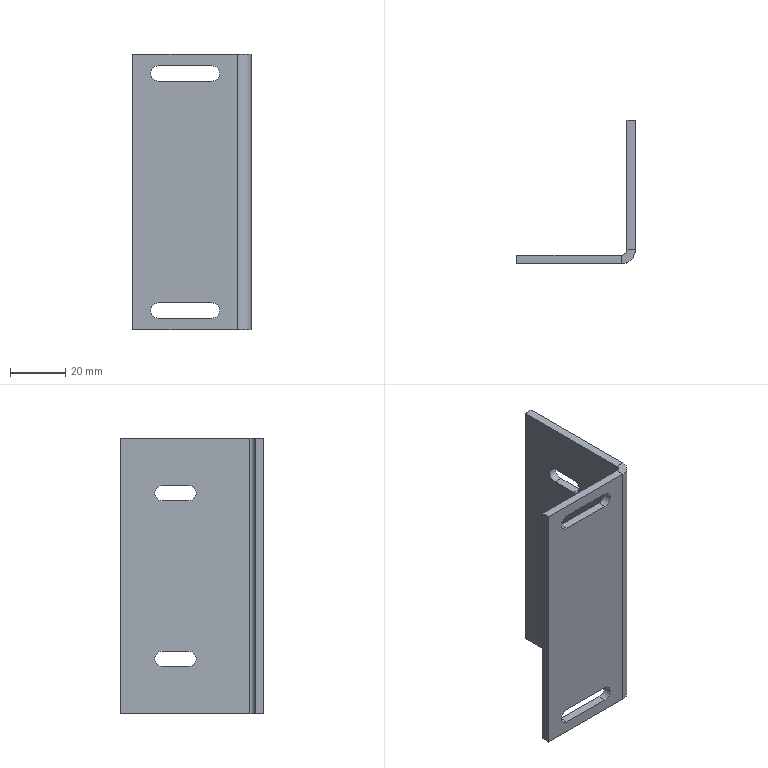Part | SolidWorks | features HoleWzd 2, FlatPattern 1, SMBaseFlange 1, SheetMetal 1 | 1 solid | 30 faces | box 43 x 52 x 100 mm | volume 25907 mm3 | plane 20 | cylinder 10 | commonest cylinder face diameters 5.5 x8 4 x1 10 x1
STEP:
#1=CARTESIAN_POINT('',(40.,2.,100.));
#2=VERTEX_POINT('',#1);
#3=CARTESIAN_POINT('',(43.,2.,100.));
#4=VERTEX_POINT('',#3);
#5=CARTESIAN_POINT('',(40.,2.,100.));
#6=DIRECTION('',(1.,0.,0.));
#7=VECTOR('',#6,1000.);
#8=LINE('',#5,#7);
#9=EDGE_CURVE('',#2,#4,#8,.T.);
#10=ORIENTED_EDGE('',*,*,#9,.F.);
#11=CARTESIAN_POINT('',(38.,0.,100.));
#12=VERTEX_POINT('',#11);
#13=CARTESIAN_POINT('',(38.,2.,100.));
#14=DIRECTION('',(0.,0.,1.));
#15=DIRECTION('',(-1.,0.,0.));
#16=AXIS2_PLACEMENT_3D('',#13,#14,#15);
#17=CIRCLE('',#16,2.);
#18=EDGE_CURVE('',#12,#2,#17,.T.);
#19=ORIENTED_EDGE('',*,*,#18,.F.);
#20=CARTESIAN_POINT('',(38.,-3.,100.));
#21=VERTEX_POINT('',#20);
#22=CARTESIAN_POINT('',(38.,-3.,100.));
#23=DIRECTION('',(0.,1.,0.));
#24=VECTOR('',#23,1000.);
#25=LINE('',#22,#24);
#26=EDGE_CURVE('',#21,#12,#25,.T.);
#27=ORIENTED_EDGE('',*,*,#26,.F.);
#28=CARTESIAN_POINT('',(38.,2.,100.));
#29=DIRECTION('',(0.,0.,1.));
#30=DIRECTION('',(1.,0.,0.));
#31=AXIS2_PLACEMENT_3D('',#28,#29,#30);
#32=CIRCLE('',#31,5.);
#33=EDGE_CURVE('',#21,#4,#32,.T.);
#34=ORIENTED_EDGE('',*,*,#33,.T.);
#35=EDGE_LOOP('',(#10,#19,#27,#34));
#36=FACE_OUTER_BOUND('',#35,.T.);
#37=CARTESIAN_POINT('',(40.,2.,100.));
#38=DIRECTION('',(0.,0.,1.));
#39=DIRECTION('',(1.,0.,0.));
#40=AXIS2_PLACEMENT_3D('',#37,#38,#39);
#41=PLANE('',#40);
#42=ADVANCED_FACE('',(#36),#41,.T.);
#43=CARTESIAN_POINT('',(40.,49.,100.));
#44=VERTEX_POINT('',#43);
#45=CARTESIAN_POINT('',(40.,0.,100.));
#46=DIRECTION('',(0.,1.,0.));
#47=VECTOR('',#46,1000.);
#48=LINE('',#45,#47);
#49=EDGE_CURVE('',#2,#44,#48,.T.);
#50=ORIENTED_EDGE('',*,*,#49,.F.);
#51=ORIENTED_EDGE('',*,*,#9,.T.);
#52=CARTESIAN_POINT('',(43.,49.,100.));
#53=VERTEX_POINT('',#52);
#54=CARTESIAN_POINT('',(43.,0.,100.));
#55=DIRECTION('',(0.,1.,0.));
#56=VECTOR('',#55,1000.);
#57=LINE('',#54,#56);
#58=EDGE_CURVE('',#4,#53,#57,.T.);
#59=ORIENTED_EDGE('',*,*,#58,.T.);
#60=CARTESIAN_POINT('',(40.,49.,100.));
#61=DIRECTION('',(1.,0.,0.));
#62=VECTOR('',#61,1000.);
#63=LINE('',#60,#62);
#64=EDGE_CURVE('',#44,#53,#63,.T.);
#65=ORIENTED_EDGE('',*,*,#64,.F.);
#66=EDGE_LOOP('',(#50,#51,#59,#65));
#67=FACE_OUTER_BOUND('',#66,.T.);
#68=CARTESIAN_POINT('',(38.,-3.,100.));
#69=DIRECTION('',(0.,0.,1.));
#70=DIRECTION('',(1.,0.,0.));
#71=AXIS2_PLACEMENT_3D('',#68,#69,#70);
#72=PLANE('',#71);
#73=ADVANCED_FACE('',(#67),#72,.T.);
#74=CARTESIAN_POINT('',(38.,0.,0.));
#75=VERTEX_POINT('',#74);
#76=CARTESIAN_POINT('',(38.,-3.,0.));
#77=VERTEX_POINT('',#76);
#78=CARTESIAN_POINT('',(38.,0.,0.));
#79=DIRECTION('',(0.,-1.,0.));
#80=VECTOR('',#79,1000.);
#81=LINE('',#78,#80);
#82=EDGE_CURVE('',#75,#77,#81,.T.);
#83=ORIENTED_EDGE('',*,*,#82,.F.);
#84=CARTESIAN_POINT('',(40.,2.,0.));
#85=VERTEX_POINT('',#84);
#86=CARTESIAN_POINT('',(38.,2.,0.));
#87=DIRECTION('',(0.,0.,1.));
#88=DIRECTION('',(-1.,0.,0.));
#89=AXIS2_PLACEMENT_3D('',#86,#87,#88);
#90=CIRCLE('',#89,2.);
#91=EDGE_CURVE('',#75,#85,#90,.T.);
#92=ORIENTED_EDGE('',*,*,#91,.T.);
#93=CARTESIAN_POINT('',(43.,2.,0.));
#94=VERTEX_POINT('',#93);
#95=CARTESIAN_POINT('',(43.,2.,0.));
#96=DIRECTION('',(-1.,0.,0.));
#97=VECTOR('',#96,1000.);
#98=LINE('',#95,#97);
#99=EDGE_CURVE('',#94,#85,#98,.T.);
#100=ORIENTED_EDGE('',*,*,#99,.F.);
#101=CARTESIAN_POINT('',(38.,2.,0.));
#102=DIRECTION('',(0.,0.,1.));
#103=DIRECTION('',(1.,0.,0.));
#104=AXIS2_PLACEMENT_3D('',#101,#102,#103);
#105=CIRCLE('',#104,5.);
#106=EDGE_CURVE('',#77,#94,#105,.T.);
#107=ORIENTED_EDGE('',*,*,#106,.F.);
#108=EDGE_LOOP('',(#83,#92,#100,#107));
#109=FACE_OUTER_BOUND('',#108,.T.);
#110=CARTESIAN_POINT('',(38.,0.,0.));
#111=DIRECTION('',(0.,0.,-1.));
#112=DIRECTION('',(-1.,0.,0.));
#113=AXIS2_PLACEMENT_3D('',#110,#111,#112);
#114=PLANE('',#113);
#115=ADVANCED_FACE('',(#109),#114,.T.);
#116=CARTESIAN_POINT('',(0.,0.,0.));
#117=VERTEX_POINT('',#116);
#118=CARTESIAN_POINT('',(0.,0.,0.));
#119=DIRECTION('',(1.,0.,0.));
#120=VECTOR('',#119,1000.);
#121=LINE('',#118,#120);
#122=EDGE_CURVE('',#117,#75,#121,.T.);
#123=ORIENTED_EDGE('',*,*,#122,.T.);
#124=ORIENTED_EDGE('',*,*,#82,.T.);
#125=CARTESIAN_POINT('',(0.,-3.,0.));
#126=VERTEX_POINT('',#125);
#127=CARTESIAN_POINT('',(0.,-3.,0.));
#128=DIRECTION('',(1.,0.,0.));
#129=VECTOR('',#128,1000.);
#130=LINE('',#127,#129);
#131=EDGE_CURVE('',#126,#77,#130,.T.);
#132=ORIENTED_EDGE('',*,*,#131,.F.);
#133=CARTESIAN_POINT('',(0.,-3.,0.));
#134=DIRECTION('',(0.,1.,0.));
#135=VECTOR('',#134,1000.);
#136=LINE('',#133,#135);
#137=EDGE_CURVE('',#126,#117,#136,.T.);
#138=ORIENTED_EDGE('',*,*,#137,.T.);
#139=EDGE_LOOP('',(#123,#124,#132,#138));
#140=FACE_OUTER_BOUND('',#139,.T.);
#141=CARTESIAN_POINT('',(43.,2.,0.));
#142=DIRECTION('',(0.,0.,-1.));
#143=DIRECTION('',(-1.,0.,0.));
#144=AXIS2_PLACEMENT_3D('',#141,#142,#143);
#145=PLANE('',#144);
#146=ADVANCED_FACE('',(#140),#145,.T.);
#147=CARTESIAN_POINT('',(43.,24.25,17.25));
#148=VERTEX_POINT('',#147);
#149=CARTESIAN_POINT('',(43.,24.25,22.75));
#150=VERTEX_POINT('',#149);
#151=CARTESIAN_POINT('',(43.,24.25,20.));
#152=DIRECTION('',(-1.,0.,0.));
#153=DIRECTION('',(0.,0.,1.));
#154=AXIS2_PLACEMENT_3D('',#151,#152,#153);
#155=CIRCLE('',#154,2.75);
#156=EDGE_CURVE('',#148,#150,#155,.T.);
#157=ORIENTED_EDGE('',*,*,#156,.T.);
#158=CARTESIAN_POINT('',(43.,33.75,22.75));
#159=VERTEX_POINT('',#158);
#160=CARTESIAN_POINT('',(43.,24.25,22.75));
#161=DIRECTION('',(0.,1.,0.));
#162=VECTOR('',#161,1000.);
#163=LINE('',#160,#162);
#164=EDGE_CURVE('',#150,#159,#163,.T.);
#165=ORIENTED_EDGE('',*,*,#164,.T.);
#166=CARTESIAN_POINT('',(43.,33.75,17.25));
#167=VERTEX_POINT('',#166);
#168=CARTESIAN_POINT('',(43.,33.75,20.));
#169=DIRECTION('',(-1.,0.,0.));
#170=DIRECTION('',(0.,0.,1.));
#171=AXIS2_PLACEMENT_3D('',#168,#169,#170);
#172=CIRCLE('',#171,2.75);
#173=EDGE_CURVE('',#159,#167,#172,.T.);
#174=ORIENTED_EDGE('',*,*,#173,.T.);
#175=CARTESIAN_POINT('',(43.,24.25,17.25));
#176=DIRECTION('',(0.,1.,0.));
#177=VECTOR('',#176,1000.);
#178=LINE('',#175,#177);
#179=EDGE_CURVE('',#148,#167,#178,.T.);
#180=ORIENTED_EDGE('',*,*,#179,.F.);
#181=EDGE_LOOP('',(#157,#165,#174,#180));
#182=FACE_BOUND('',#181,.T.);
#183=CARTESIAN_POINT('',(43.,33.75,82.75));
#184=VERTEX_POINT('',#183);
#185=CARTESIAN_POINT('',(43.,33.75,77.25));
#186=VERTEX_POINT('',#185);
#187=CARTESIAN_POINT('',(43.,33.75,80.));
#188=DIRECTION('',(-1.,0.,0.));
#189=DIRECTION('',(0.,0.,1.));
#190=AXIS2_PLACEMENT_3D('',#187,#188,#189);
#191=CIRCLE('',#190,2.75);
#192=EDGE_CURVE('',#184,#186,#191,.T.);
#193=ORIENTED_EDGE('',*,*,#192,.T.);
#194=CARTESIAN_POINT('',(43.,24.25,77.25));
#195=VERTEX_POINT('',#194);
#196=CARTESIAN_POINT('',(43.,24.25,77.25));
#197=DIRECTION('',(0.,1.,0.));
#198=VECTOR('',#197,1000.);
#199=LINE('',#196,#198);
#200=EDGE_CURVE('',#195,#186,#199,.T.);
#201=ORIENTED_EDGE('',*,*,#200,.F.);
#202=CARTESIAN_POINT('',(43.,24.25,82.75));
#203=VERTEX_POINT('',#202);
#204=CARTESIAN_POINT('',(43.,24.25,80.));
#205=DIRECTION('',(-1.,0.,0.));
#206=DIRECTION('',(0.,0.,1.));
#207=AXIS2_PLACEMENT_3D('',#204,#205,#206);
#208=CIRCLE('',#207,2.75);
#209=EDGE_CURVE('',#195,#203,#208,.T.);
#210=ORIENTED_EDGE('',*,*,#209,.T.);
#211=CARTESIAN_POINT('',(43.,24.25,82.75));
#212=DIRECTION('',(0.,1.,0.));
#213=VECTOR('',#212,1000.);
#214=LINE('',#211,#213);
#215=EDGE_CURVE('',#203,#184,#214,.T.);
#216=ORIENTED_EDGE('',*,*,#215,.T.);
#217=EDGE_LOOP('',(#193,#201,#210,#216));
#218=FACE_BOUND('',#217,.T.);
#219=CARTESIAN_POINT('',(43.,49.,0.));
#220=VERTEX_POINT('',#219);
#221=CARTESIAN_POINT('',(43.,0.,0.));
#222=DIRECTION('',(0.,1.,0.));
#223=VECTOR('',#222,1000.);
#224=LINE('',#221,#223);
#225=EDGE_CURVE('',#94,#220,#224,.T.);
#226=ORIENTED_EDGE('',*,*,#225,.T.);
#227=CARTESIAN_POINT('',(43.,49.,100.));
#228=DIRECTION('',(0.,0.,-1.));
#229=VECTOR('',#228,1000.);
#230=LINE('',#227,#229);
#231=EDGE_CURVE('',#53,#220,#230,.T.);
#232=ORIENTED_EDGE('',*,*,#231,.F.);
#233=ORIENTED_EDGE('',*,*,#58,.F.);
#234=CARTESIAN_POINT('',(43.,2.,100.));
#235=DIRECTION('',(0.,0.,-1.));
#236=VECTOR('',#235,1000.);
#237=LINE('',#234,#236);
#238=EDGE_CURVE('',#4,#94,#237,.T.);
#239=ORIENTED_EDGE('',*,*,#238,.T.);
#240=EDGE_LOOP('',(#226,#232,#233,#239));
#241=FACE_OUTER_BOUND('',#240,.T.);
#242=CARTESIAN_POINT('',(43.,0.,100.));
#243=DIRECTION('',(-1.,0.,0.));
#244=DIRECTION('',(0.,0.,1.));
#245=AXIS2_PLACEMENT_3D('',#242,#243,#244);
#246=PLANE('',#245);
#247=ADVANCED_FACE('',(#182,#218,#241),#246,.F.);
#248=CARTESIAN_POINT('',(40.,49.,0.));
#249=VERTEX_POINT('',#248);
#250=CARTESIAN_POINT('',(40.,49.,0.));
#251=DIRECTION('',(1.,0.,0.));
#252=VECTOR('',#251,1000.);
#253=LINE('',#250,#252);
#254=EDGE_CURVE('',#249,#220,#253,.T.);
#255=ORIENTED_EDGE('',*,*,#254,.F.);
#256=CARTESIAN_POINT('',(40.,49.,100.));
#257=DIRECTION('',(0.,0.,-1.));
#258=VECTOR('',#257,1000.);
#259=LINE('',#256,#258);
#260=EDGE_CURVE('',#44,#249,#259,.T.);
#261=ORIENTED_EDGE('',*,*,#260,.F.);
#262=ORIENTED_EDGE('',*,*,#64,.T.);
#263=ORIENTED_EDGE('',*,*,#231,.T.);
#264=EDGE_LOOP('',(#255,#261,#262,#263));
#265=FACE_OUTER_BOUND('',#264,.T.);
#266=CARTESIAN_POINT('',(40.,49.,100.));
#267=DIRECTION('',(0.,1.,0.));
#268=DIRECTION('',(0.,0.,1.));
#269=AXIS2_PLACEMENT_3D('',#266,#267,#268);
#270=PLANE('',#269);
#271=ADVANCED_FACE('',(#265),#270,.T.);
#272=CARTESIAN_POINT('',(40.,33.75,22.75));
#273=VERTEX_POINT('',#272);
#274=CARTESIAN_POINT('',(40.,33.75,17.25));
#275=VERTEX_POINT('',#274);
#276=CARTESIAN_POINT('',(40.,33.75,20.));
#277=DIRECTION('',(-1.,0.,0.));
#278=DIRECTION('',(0.,0.,1.));
#279=AXIS2_PLACEMENT_3D('',#276,#277,#278);
#280=CIRCLE('',#279,2.75);
#281=EDGE_CURVE('',#273,#275,#280,.T.);
#282=ORIENTED_EDGE('',*,*,#281,.F.);
#283=CARTESIAN_POINT('',(40.,24.25,22.75));
#284=VERTEX_POINT('',#283);
#285=CARTESIAN_POINT('',(40.,24.25,22.75));
#286=DIRECTION('',(0.,1.,0.));
#287=VECTOR('',#286,1000.);
#288=LINE('',#285,#287);
#289=EDGE_CURVE('',#284,#273,#288,.T.);
#290=ORIENTED_EDGE('',*,*,#289,.F.);
#291=CARTESIAN_POINT('',(40.,24.25,17.25));
#292=VERTEX_POINT('',#291);
#293=CARTESIAN_POINT('',(40.,24.25,20.));
#294=DIRECTION('',(-1.,0.,0.));
#295=DIRECTION('',(0.,0.,1.));
#296=AXIS2_PLACEMENT_3D('',#293,#294,#295);
#297=CIRCLE('',#296,2.75);
#298=EDGE_CURVE('',#292,#284,#297,.T.);
#299=ORIENTED_EDGE('',*,*,#298,.F.);
#300=CARTESIAN_POINT('',(40.,24.25,17.25));
#301=DIRECTION('',(0.,1.,0.));
#302=VECTOR('',#301,1000.);
#303=LINE('',#300,#302);
#304=EDGE_CURVE('',#292,#275,#303,.T.);
#305=ORIENTED_EDGE('',*,*,#304,.T.);
#306=EDGE_LOOP('',(#282,#290,#299,#305));
#307=FACE_BOUND('',#306,.T.);
#308=CARTESIAN_POINT('',(40.,33.75,82.75));
#309=VERTEX_POINT('',#308);
#310=CARTESIAN_POINT('',(40.,33.75,77.25));
#311=VERTEX_POINT('',#310);
#312=CARTESIAN_POINT('',(40.,33.75,80.));
#313=DIRECTION('',(-1.,0.,0.));
#314=DIRECTION('',(0.,0.,1.));
#315=AXIS2_PLACEMENT_3D('',#312,#313,#314);
#316=CIRCLE('',#315,2.75);
#317=EDGE_CURVE('',#309,#311,#316,.T.);
#318=ORIENTED_EDGE('',*,*,#317,.F.);
#319=CARTESIAN_POINT('',(40.,24.25,82.75));
#320=VERTEX_POINT('',#319);
#321=CARTESIAN_POINT('',(40.,24.25,82.75));
#322=DIRECTION('',(0.,1.,0.));
#323=VECTOR('',#322,1000.);
#324=LINE('',#321,#323);
#325=EDGE_CURVE('',#320,#309,#324,.T.);
#326=ORIENTED_EDGE('',*,*,#325,.F.);
#327=CARTESIAN_POINT('',(40.,24.25,77.25));
#328=VERTEX_POINT('',#327);
#329=CARTESIAN_POINT('',(40.,24.25,80.));
#330=DIRECTION('',(-1.,0.,0.));
#331=DIRECTION('',(0.,0.,1.));
#332=AXIS2_PLACEMENT_3D('',#329,#330,#331);
#333=CIRCLE('',#332,2.75);
#334=EDGE_CURVE('',#328,#320,#333,.T.);
#335=ORIENTED_EDGE('',*,*,#334,.F.);
#336=CARTESIAN_POINT('',(40.,24.25,77.25));
#337=DIRECTION('',(0.,1.,0.));
#338=VECTOR('',#337,1000.);
#339=LINE('',#336,#338);
#340=EDGE_CURVE('',#328,#311,#339,.T.);
#341=ORIENTED_EDGE('',*,*,#340,.T.);
#342=EDGE_LOOP('',(#318,#326,#335,#341));
#343=FACE_BOUND('',#342,.T.);
#344=CARTESIAN_POINT('',(40.,0.,0.));
#345=DIRECTION('',(0.,1.,0.));
#346=VECTOR('',#345,1000.);
#347=LINE('',#344,#346);
#348=EDGE_CURVE('',#85,#249,#347,.T.);
#349=ORIENTED_EDGE('',*,*,#348,.F.);
#350=CARTESIAN_POINT('',(40.,2.,100.));
#351=DIRECTION('',(0.,0.,-1.));
#352=VECTOR('',#351,1000.);
#353=LINE('',#350,#352);
#354=EDGE_CURVE('',#2,#85,#353,.T.);
#355=ORIENTED_EDGE('',*,*,#354,.F.);
#356=ORIENTED_EDGE('',*,*,#49,.T.);
#357=ORIENTED_EDGE('',*,*,#260,.T.);
#358=EDGE_LOOP('',(#349,#355,#356,#357));
#359=FACE_OUTER_BOUND('',#358,.T.);
#360=CARTESIAN_POINT('',(40.,0.,100.));
#361=DIRECTION('',(-1.,0.,0.));
#362=DIRECTION('',(0.,0.,1.));
#363=AXIS2_PLACEMENT_3D('',#360,#361,#362);
#364=PLANE('',#363);
#365=ADVANCED_FACE('',(#307,#343,#359),#364,.T.);
#366=ORIENTED_EDGE('',*,*,#91,.F.);
#367=CARTESIAN_POINT('',(38.,0.,100.));
#368=DIRECTION('',(0.,0.,-1.));
#369=VECTOR('',#368,1000.);
#370=LINE('',#367,#369);
#371=EDGE_CURVE('',#12,#75,#370,.T.);
#372=ORIENTED_EDGE('',*,*,#371,.F.);
#373=ORIENTED_EDGE('',*,*,#18,.T.);
#374=ORIENTED_EDGE('',*,*,#354,.T.);
#375=EDGE_LOOP('',(#366,#372,#373,#374));
#376=FACE_OUTER_BOUND('',#375,.T.);
#377=CARTESIAN_POINT('',(38.,2.,100.));
#378=DIRECTION('',(0.,0.,-1.));
#379=DIRECTION('',(-1.,0.,0.));
#380=AXIS2_PLACEMENT_3D('',#377,#378,#379);
#381=CYLINDRICAL_SURFACE('',#380,2.);
#382=ADVANCED_FACE('',(#376),#381,.F.);
#383=CARTESIAN_POINT('',(9.25,0.,9.75));
#384=VERTEX_POINT('',#383);
#385=CARTESIAN_POINT('',(28.75,0.,9.75));
#386=VERTEX_POINT('',#385);
#387=CARTESIAN_POINT('',(9.25,0.,9.75));
#388=DIRECTION('',(1.,0.,0.));
#389=VECTOR('',#388,1000.);
#390=LINE('',#387,#389);
#391=EDGE_CURVE('',#384,#386,#390,.T.);
#392=ORIENTED_EDGE('',*,*,#391,.F.);
#393=CARTESIAN_POINT('',(9.25,0.,4.25));
#394=VERTEX_POINT('',#393);
#395=CARTESIAN_POINT('',(9.25,0.,7.));
#396=DIRECTION('',(0.,1.,0.));
#397=DIRECTION('',(0.,0.,1.));
#398=AXIS2_PLACEMENT_3D('',#395,#396,#397);
#399=CIRCLE('',#398,2.75);
#400=EDGE_CURVE('',#394,#384,#399,.T.);
#401=ORIENTED_EDGE('',*,*,#400,.F.);
#402=CARTESIAN_POINT('',(28.75,0.,4.25));
#403=VERTEX_POINT('',#402);
#404=CARTESIAN_POINT('',(9.25,0.,4.25));
#405=DIRECTION('',(1.,0.,0.));
#406=VECTOR('',#405,1000.);
#407=LINE('',#404,#406);
#408=EDGE_CURVE('',#394,#403,#407,.T.);
#409=ORIENTED_EDGE('',*,*,#408,.T.);
#410=CARTESIAN_POINT('',(28.75,0.,7.));
#411=DIRECTION('',(0.,1.,0.));
#412=DIRECTION('',(0.,0.,1.));
#413=AXIS2_PLACEMENT_3D('',#410,#411,#412);
#414=CIRCLE('',#413,2.75);
#415=EDGE_CURVE('',#386,#403,#414,.T.);
#416=ORIENTED_EDGE('',*,*,#415,.F.);
#417=EDGE_LOOP('',(#392,#401,#409,#416));
#418=FACE_BOUND('',#417,.T.);
#419=CARTESIAN_POINT('',(9.25,0.,90.25));
#420=VERTEX_POINT('',#419);
#421=CARTESIAN_POINT('',(9.25,0.,95.75));
#422=VERTEX_POINT('',#421);
#423=CARTESIAN_POINT('',(9.25,0.,93.));
#424=DIRECTION('',(0.,1.,0.));
#425=DIRECTION('',(0.,0.,1.));
#426=AXIS2_PLACEMENT_3D('',#423,#424,#425);
#427=CIRCLE('',#426,2.75);
#428=EDGE_CURVE('',#420,#422,#427,.T.);
#429=ORIENTED_EDGE('',*,*,#428,.F.);
#430=CARTESIAN_POINT('',(28.75,0.,90.25));
#431=VERTEX_POINT('',#430);
#432=CARTESIAN_POINT('',(9.25,0.,90.25));
#433=DIRECTION('',(1.,0.,0.));
#434=VECTOR('',#433,1000.);
#435=LINE('',#432,#434);
#436=EDGE_CURVE('',#420,#431,#435,.T.);
#437=ORIENTED_EDGE('',*,*,#436,.T.);
#438=CARTESIAN_POINT('',(28.75,0.,95.75));
#439=VERTEX_POINT('',#438);
#440=CARTESIAN_POINT('',(28.75,0.,93.));
#441=DIRECTION('',(0.,1.,0.));
#442=DIRECTION('',(0.,0.,1.));
#443=AXIS2_PLACEMENT_3D('',#440,#441,#442);
#444=CIRCLE('',#443,2.75);
#445=EDGE_CURVE('',#439,#431,#444,.T.);
#446=ORIENTED_EDGE('',*,*,#445,.F.);
#447=CARTESIAN_POINT('',(9.25,0.,95.75));
#448=DIRECTION('',(1.,0.,0.));
#449=VECTOR('',#448,1000.);
#450=LINE('',#447,#449);
#451=EDGE_CURVE('',#422,#439,#450,.T.);
#452=ORIENTED_EDGE('',*,*,#451,.F.);
#453=EDGE_LOOP('',(#429,#437,#446,#452));
#454=FACE_BOUND('',#453,.T.);
#455=ORIENTED_EDGE('',*,*,#122,.F.);
#456=CARTESIAN_POINT('',(0.,0.,100.));
#457=VERTEX_POINT('',#456);
#458=CARTESIAN_POINT('',(0.,0.,100.));
#459=DIRECTION('',(0.,0.,-1.));
#460=VECTOR('',#459,1000.);
#461=LINE('',#458,#460);
#462=EDGE_CURVE('',#457,#117,#461,.T.);
#463=ORIENTED_EDGE('',*,*,#462,.F.);
#464=CARTESIAN_POINT('',(0.,0.,100.));
#465=DIRECTION('',(1.,0.,0.));
#466=VECTOR('',#465,1000.);
#467=LINE('',#464,#466);
#468=EDGE_CURVE('',#457,#12,#467,.T.);
#469=ORIENTED_EDGE('',*,*,#468,.T.);
#470=ORIENTED_EDGE('',*,*,#371,.T.);
#471=EDGE_LOOP('',(#455,#463,#469,#470));
#472=FACE_OUTER_BOUND('',#471,.T.);
#473=CARTESIAN_POINT('',(0.,0.,100.));
#474=DIRECTION('',(0.,1.,0.));
#475=DIRECTION('',(0.,0.,1.));
#476=AXIS2_PLACEMENT_3D('',#473,#474,#475);
#477=PLANE('',#476);
#478=ADVANCED_FACE('',(#418,#454,#472),#477,.T.);
#479=ORIENTED_EDGE('',*,*,#137,.F.);
#480=CARTESIAN_POINT('',(0.,-3.,100.));
#481=VERTEX_POINT('',#480);
#482=CARTESIAN_POINT('',(0.,-3.,100.));
#483=DIRECTION('',(0.,0.,-1.));
#484=VECTOR('',#483,1000.);
#485=LINE('',#482,#484);
#486=EDGE_CURVE('',#481,#126,#485,.T.);
#487=ORIENTED_EDGE('',*,*,#486,.F.);
#488=CARTESIAN_POINT('',(0.,-3.,100.));
#489=DIRECTION('',(0.,1.,0.));
#490=VECTOR('',#489,1000.);
#491=LINE('',#488,#490);
#492=EDGE_CURVE('',#481,#457,#491,.T.);
#493=ORIENTED_EDGE('',*,*,#492,.T.);
#494=ORIENTED_EDGE('',*,*,#462,.T.);
#495=EDGE_LOOP('',(#479,#487,#493,#494));
#496=FACE_OUTER_BOUND('',#495,.T.);
#497=CARTESIAN_POINT('',(0.,-3.,100.));
#498=DIRECTION('',(-1.,0.,0.));
#499=DIRECTION('',(0.,0.,1.));
#500=AXIS2_PLACEMENT_3D('',#497,#498,#499);
#501=PLANE('',#500);
#502=ADVANCED_FACE('',(#496),#501,.T.);
#503=CARTESIAN_POINT('',(9.25,-3.,9.75));
#504=VERTEX_POINT('',#503);
#505=CARTESIAN_POINT('',(28.75,-3.,9.75));
#506=VERTEX_POINT('',#505);
#507=CARTESIAN_POINT('',(9.25,-3.,9.75));
#508=DIRECTION('',(1.,0.,0.));
#509=VECTOR('',#508,1000.);
#510=LINE('',#507,#509);
#511=EDGE_CURVE('',#504,#506,#510,.T.);
#512=ORIENTED_EDGE('',*,*,#511,.T.);
#513=CARTESIAN_POINT('',(28.75,-3.,4.25));
#514=VERTEX_POINT('',#513);
#515=CARTESIAN_POINT('',(28.75,-3.,7.));
#516=DIRECTION('',(0.,1.,0.));
#517=DIRECTION('',(0.,0.,1.));
#518=AXIS2_PLACEMENT_3D('',#515,#516,#517);
#519=CIRCLE('',#518,2.75);
#520=EDGE_CURVE('',#506,#514,#519,.T.);
#521=ORIENTED_EDGE('',*,*,#520,.T.);
#522=CARTESIAN_POINT('',(9.25,-3.,4.25));
#523=VERTEX_POINT('',#522);
#524=CARTESIAN_POINT('',(9.25,-3.,4.25));
#525=DIRECTION('',(1.,0.,0.));
#526=VECTOR('',#525,1000.);
#527=LINE('',#524,#526);
#528=EDGE_CURVE('',#523,#514,#527,.T.);
#529=ORIENTED_EDGE('',*,*,#528,.F.);
#530=CARTESIAN_POINT('',(9.25,-3.,7.));
#531=DIRECTION('',(0.,1.,0.));
#532=DIRECTION('',(0.,0.,1.));
#533=AXIS2_PLACEMENT_3D('',#530,#531,#532);
#534=CIRCLE('',#533,2.75);
#535=EDGE_CURVE('',#523,#504,#534,.T.);
#536=ORIENTED_EDGE('',*,*,#535,.T.);
#537=EDGE_LOOP('',(#512,#521,#529,#536));
#538=FACE_BOUND('',#537,.T.);
#539=CARTESIAN_POINT('',(9.25,-3.,90.25));
#540=VERTEX_POINT('',#539);
#541=CARTESIAN_POINT('',(9.25,-3.,95.75));
#542=VERTEX_POINT('',#541);
#543=CARTESIAN_POINT('',(9.25,-3.,93.));
#544=DIRECTION('',(0.,1.,0.));
#545=DIRECTION('',(0.,0.,1.));
#546=AXIS2_PLACEMENT_3D('',#543,#544,#545);
#547=CIRCLE('',#546,2.75);
#548=EDGE_CURVE('',#540,#542,#547,.T.);
#549=ORIENTED_EDGE('',*,*,#548,.T.);
#550=CARTESIAN_POINT('',(28.75,-3.,95.75));
#551=VERTEX_POINT('',#550);
#552=CARTESIAN_POINT('',(9.25,-3.,95.75));
#553=DIRECTION('',(1.,0.,0.));
#554=VECTOR('',#553,1000.);
#555=LINE('',#552,#554);
#556=EDGE_CURVE('',#542,#551,#555,.T.);
#557=ORIENTED_EDGE('',*,*,#556,.T.);
#558=CARTESIAN_POINT('',(28.75,-3.,90.25));
#559=VERTEX_POINT('',#558);
#560=CARTESIAN_POINT('',(28.75,-3.,93.));
#561=DIRECTION('',(0.,1.,0.));
#562=DIRECTION('',(0.,0.,1.));
#563=AXIS2_PLACEMENT_3D('',#560,#561,#562);
#564=CIRCLE('',#563,2.75);
#565=EDGE_CURVE('',#551,#559,#564,.T.);
#566=ORIENTED_EDGE('',*,*,#565,.T.);
#567=CARTESIAN_POINT('',(9.25,-3.,90.25));
#568=DIRECTION('',(1.,0.,0.));
#569=VECTOR('',#568,1000.);
#570=LINE('',#567,#569);
#571=EDGE_CURVE('',#540,#559,#570,.T.);
#572=ORIENTED_EDGE('',*,*,#571,.F.);
#573=EDGE_LOOP('',(#549,#557,#566,#572));
#574=FACE_BOUND('',#573,.T.);
#575=ORIENTED_EDGE('',*,*,#131,.T.);
#576=CARTESIAN_POINT('',(38.,-3.,100.));
#577=DIRECTION('',(0.,0.,-1.));
#578=VECTOR('',#577,1000.);
#579=LINE('',#576,#578);
#580=EDGE_CURVE('',#21,#77,#579,.T.);
#581=ORIENTED_EDGE('',*,*,#580,.F.);
#582=CARTESIAN_POINT('',(0.,-3.,100.));
#583=DIRECTION('',(1.,0.,0.));
#584=VECTOR('',#583,1000.);
#585=LINE('',#582,#584);
#586=EDGE_CURVE('',#481,#21,#585,.T.);
#587=ORIENTED_EDGE('',*,*,#586,.F.);
#588=ORIENTED_EDGE('',*,*,#486,.T.);
#589=EDGE_LOOP('',(#575,#581,#587,#588));
#590=FACE_OUTER_BOUND('',#589,.T.);
#591=CARTESIAN_POINT('',(0.,-3.,100.));
#592=DIRECTION('',(0.,1.,0.));
#593=DIRECTION('',(0.,0.,1.));
#594=AXIS2_PLACEMENT_3D('',#591,#592,#593);
#595=PLANE('',#594);
#596=ADVANCED_FACE('',(#538,#574,#590),#595,.F.);
#597=ORIENTED_EDGE('',*,*,#106,.T.);
#598=ORIENTED_EDGE('',*,*,#238,.F.);
#599=ORIENTED_EDGE('',*,*,#33,.F.);
#600=ORIENTED_EDGE('',*,*,#580,.T.);
#601=EDGE_LOOP('',(#597,#598,#599,#600));
#602=FACE_OUTER_BOUND('',#601,.T.);
#603=CARTESIAN_POINT('',(38.,2.,100.));
#604=DIRECTION('',(0.,0.,-1.));
#605=DIRECTION('',(-1.,0.,0.));
#606=AXIS2_PLACEMENT_3D('',#603,#604,#605);
#607=CYLINDRICAL_SURFACE('',#606,5.);
#608=ADVANCED_FACE('',(#602),#607,.T.);
#609=ORIENTED_EDGE('',*,*,#586,.T.);
#610=ORIENTED_EDGE('',*,*,#26,.T.);
#611=ORIENTED_EDGE('',*,*,#468,.F.);
#612=ORIENTED_EDGE('',*,*,#492,.F.);
#613=EDGE_LOOP('',(#609,#610,#611,#612));
#614=FACE_OUTER_BOUND('',#613,.T.);
#615=CARTESIAN_POINT('',(38.,2.,100.));
#616=DIRECTION('',(0.,0.,-1.));
#617=DIRECTION('',(-1.,0.,0.));
#618=AXIS2_PLACEMENT_3D('',#615,#616,#617);
#619=PLANE('',#618);
#620=ADVANCED_FACE('',(#614),#619,.F.);
#621=ORIENTED_EDGE('',*,*,#225,.F.);
#622=ORIENTED_EDGE('',*,*,#99,.T.);
#623=ORIENTED_EDGE('',*,*,#348,.T.);
#624=ORIENTED_EDGE('',*,*,#254,.T.);
#625=EDGE_LOOP('',(#621,#622,#623,#624));
#626=FACE_OUTER_BOUND('',#625,.T.);
#627=CARTESIAN_POINT('',(38.,2.,0.));
#628=DIRECTION('',(0.,0.,-1.));
#629=DIRECTION('',(-1.,0.,0.));
#630=AXIS2_PLACEMENT_3D('',#627,#628,#629);
#631=PLANE('',#630);
#632=ADVANCED_FACE('',(#626),#631,.T.);
#633=ORIENTED_EDGE('',*,*,#565,.F.);
#634=CARTESIAN_POINT('',(28.75,0.,95.75));
#635=DIRECTION('',(0.,-1.,0.));
#636=VECTOR('',#635,1000.);
#637=LINE('',#634,#636);
#638=EDGE_CURVE('',#439,#551,#637,.T.);
#639=ORIENTED_EDGE('',*,*,#638,.F.);
#640=ORIENTED_EDGE('',*,*,#445,.T.);
#641=CARTESIAN_POINT('',(28.75,0.,90.25));
#642=DIRECTION('',(0.,1.,0.));
#643=VECTOR('',#642,1000.);
#644=LINE('',#641,#643);
#645=EDGE_CURVE('',#559,#431,#644,.T.);
#646=ORIENTED_EDGE('',*,*,#645,.F.);
#647=EDGE_LOOP('',(#633,#639,#640,#646));
#648=FACE_OUTER_BOUND('',#647,.T.);
#649=CARTESIAN_POINT('',(28.75,0.,93.));
#650=DIRECTION('',(0.,1.,0.));
#651=DIRECTION('',(0.,0.,1.));
#652=AXIS2_PLACEMENT_3D('',#649,#650,#651);
#653=CYLINDRICAL_SURFACE('',#652,2.75);
#654=ADVANCED_FACE('',(#648),#653,.F.);
#655=ORIENTED_EDGE('',*,*,#428,.T.);
#656=CARTESIAN_POINT('',(9.25,0.,95.75));
#657=DIRECTION('',(0.,1.,0.));
#658=VECTOR('',#657,1000.);
#659=LINE('',#656,#658);
#660=EDGE_CURVE('',#542,#422,#659,.T.);
#661=ORIENTED_EDGE('',*,*,#660,.F.);
#662=ORIENTED_EDGE('',*,*,#548,.F.);
#663=CARTESIAN_POINT('',(9.25,0.,90.25));
#664=DIRECTION('',(0.,-1.,0.));
#665=VECTOR('',#664,1000.);
#666=LINE('',#663,#665);
#667=EDGE_CURVE('',#420,#540,#666,.T.);
#668=ORIENTED_EDGE('',*,*,#667,.F.);
#669=EDGE_LOOP('',(#655,#661,#662,#668));
#670=FACE_OUTER_BOUND('',#669,.T.);
#671=CARTESIAN_POINT('',(9.25,0.,93.));
#672=DIRECTION('',(0.,1.,0.));
#673=DIRECTION('',(0.,0.,1.));
#674=AXIS2_PLACEMENT_3D('',#671,#672,#673);
#675=CYLINDRICAL_SURFACE('',#674,2.75);
#676=ADVANCED_FACE('',(#670),#675,.F.);
#677=ORIENTED_EDGE('',*,*,#645,.T.);
#678=ORIENTED_EDGE('',*,*,#436,.F.);
#679=ORIENTED_EDGE('',*,*,#667,.T.);
#680=ORIENTED_EDGE('',*,*,#571,.T.);
#681=EDGE_LOOP('',(#677,#678,#679,#680));
#682=FACE_OUTER_BOUND('',#681,.T.);
#683=CARTESIAN_POINT('',(9.25,0.,90.25));
#684=DIRECTION('',(0.,0.,-1.));
#685=DIRECTION('',(-1.,0.,0.));
#686=AXIS2_PLACEMENT_3D('',#683,#684,#685);
#687=PLANE('',#686);
#688=ADVANCED_FACE('',(#682),#687,.F.);
#689=ORIENTED_EDGE('',*,*,#638,.T.);
#690=ORIENTED_EDGE('',*,*,#556,.F.);
#691=ORIENTED_EDGE('',*,*,#660,.T.);
#692=ORIENTED_EDGE('',*,*,#451,.T.);
#693=EDGE_LOOP('',(#689,#690,#691,#692));
#694=FACE_OUTER_BOUND('',#693,.T.);
#695=CARTESIAN_POINT('',(9.25,0.,95.75));
#696=DIRECTION('',(0.,0.,1.));
#697=DIRECTION('',(1.,0.,0.));
#698=AXIS2_PLACEMENT_3D('',#695,#696,#697);
#699=PLANE('',#698);
#700=ADVANCED_FACE('',(#694),#699,.F.);
#701=ORIENTED_EDGE('',*,*,#520,.F.);
#702=CARTESIAN_POINT('',(28.75,0.,9.75));
#703=DIRECTION('',(0.,-1.,0.));
#704=VECTOR('',#703,1000.);
#705=LINE('',#702,#704);
#706=EDGE_CURVE('',#386,#506,#705,.T.);
#707=ORIENTED_EDGE('',*,*,#706,.F.);
#708=ORIENTED_EDGE('',*,*,#415,.T.);
#709=CARTESIAN_POINT('',(28.75,0.,4.25));
#710=DIRECTION('',(0.,1.,0.));
#711=VECTOR('',#710,1000.);
#712=LINE('',#709,#711);
#713=EDGE_CURVE('',#514,#403,#712,.T.);
#714=ORIENTED_EDGE('',*,*,#713,.F.);
#715=EDGE_LOOP('',(#701,#707,#708,#714));
#716=FACE_OUTER_BOUND('',#715,.T.);
#717=CARTESIAN_POINT('',(28.75,0.,7.));
#718=DIRECTION('',(0.,1.,0.));
#719=DIRECTION('',(0.,0.,1.));
#720=AXIS2_PLACEMENT_3D('',#717,#718,#719);
#721=CYLINDRICAL_SURFACE('',#720,2.75);
#722=ADVANCED_FACE('',(#716),#721,.F.);
#723=ORIENTED_EDGE('',*,*,#400,.T.);
#724=CARTESIAN_POINT('',(9.25,0.,9.75));
#725=DIRECTION('',(0.,1.,0.));
#726=VECTOR('',#725,1000.);
#727=LINE('',#724,#726);
#728=EDGE_CURVE('',#504,#384,#727,.T.);
#729=ORIENTED_EDGE('',*,*,#728,.F.);
#730=ORIENTED_EDGE('',*,*,#535,.F.);
#731=CARTESIAN_POINT('',(9.25,0.,4.25));
#732=DIRECTION('',(0.,-1.,0.));
#733=VECTOR('',#732,1000.);
#734=LINE('',#731,#733);
#735=EDGE_CURVE('',#394,#523,#734,.T.);
#736=ORIENTED_EDGE('',*,*,#735,.F.);
#737=EDGE_LOOP('',(#723,#729,#730,#736));
#738=FACE_OUTER_BOUND('',#737,.T.);
#739=CARTESIAN_POINT('',(9.25,0.,7.));
#740=DIRECTION('',(0.,1.,0.));
#741=DIRECTION('',(0.,0.,1.));
#742=AXIS2_PLACEMENT_3D('',#739,#740,#741);
#743=CYLINDRICAL_SURFACE('',#742,2.75);
#744=ADVANCED_FACE('',(#738),#743,.F.);
#745=ORIENTED_EDGE('',*,*,#713,.T.);
#746=ORIENTED_EDGE('',*,*,#408,.F.);
#747=ORIENTED_EDGE('',*,*,#735,.T.);
#748=ORIENTED_EDGE('',*,*,#528,.T.);
#749=EDGE_LOOP('',(#745,#746,#747,#748));
#750=FACE_OUTER_BOUND('',#749,.T.);
#751=CARTESIAN_POINT('',(9.25,0.,4.25));
#752=DIRECTION('',(0.,0.,-1.));
#753=DIRECTION('',(-1.,0.,0.));
#754=AXIS2_PLACEMENT_3D('',#751,#752,#753);
#755=PLANE('',#754);
#756=ADVANCED_FACE('',(#750),#755,.F.);
#757=ORIENTED_EDGE('',*,*,#706,.T.);
#758=ORIENTED_EDGE('',*,*,#511,.F.);
#759=ORIENTED_EDGE('',*,*,#728,.T.);
#760=ORIENTED_EDGE('',*,*,#391,.T.);
#761=EDGE_LOOP('',(#757,#758,#759,#760));
#762=FACE_OUTER_BOUND('',#761,.T.);
#763=CARTESIAN_POINT('',(9.25,0.,9.75));
#764=DIRECTION('',(0.,0.,1.));
#765=DIRECTION('',(1.,0.,0.));
#766=AXIS2_PLACEMENT_3D('',#763,#764,#765);
#767=PLANE('',#766);
#768=ADVANCED_FACE('',(#762),#767,.F.);
#769=ORIENTED_EDGE('',*,*,#192,.F.);
#770=CARTESIAN_POINT('',(40.,33.75,82.75));
#771=DIRECTION('',(1.,0.,0.));
#772=VECTOR('',#771,1000.);
#773=LINE('',#770,#772);
#774=EDGE_CURVE('',#309,#184,#773,.T.);
#775=ORIENTED_EDGE('',*,*,#774,.F.);
#776=ORIENTED_EDGE('',*,*,#317,.T.);
#777=CARTESIAN_POINT('',(40.,33.75,77.25));
#778=DIRECTION('',(-1.,0.,0.));
#779=VECTOR('',#778,1000.);
#780=LINE('',#777,#779);
#781=EDGE_CURVE('',#186,#311,#780,.T.);
#782=ORIENTED_EDGE('',*,*,#781,.F.);
#783=EDGE_LOOP('',(#769,#775,#776,#782));
#784=FACE_OUTER_BOUND('',#783,.T.);
#785=CARTESIAN_POINT('',(40.,33.75,80.));
#786=DIRECTION('',(-1.,0.,0.));
#787=DIRECTION('',(0.,0.,1.));
#788=AXIS2_PLACEMENT_3D('',#785,#786,#787);
#789=CYLINDRICAL_SURFACE('',#788,2.75);
#790=ADVANCED_FACE('',(#784),#789,.F.);
#791=ORIENTED_EDGE('',*,*,#334,.T.);
#792=CARTESIAN_POINT('',(40.,24.25,82.75));
#793=DIRECTION('',(-1.,0.,0.));
#794=VECTOR('',#793,1000.);
#795=LINE('',#792,#794);
#796=EDGE_CURVE('',#203,#320,#795,.T.);
#797=ORIENTED_EDGE('',*,*,#796,.F.);
#798=ORIENTED_EDGE('',*,*,#209,.F.);
#799=CARTESIAN_POINT('',(40.,24.25,77.25));
#800=DIRECTION('',(1.,0.,0.));
#801=VECTOR('',#800,1000.);
#802=LINE('',#799,#801);
#803=EDGE_CURVE('',#328,#195,#802,.T.);
#804=ORIENTED_EDGE('',*,*,#803,.F.);
#805=EDGE_LOOP('',(#791,#797,#798,#804));
#806=FACE_OUTER_BOUND('',#805,.T.);
#807=CARTESIAN_POINT('',(40.,24.25,80.));
#808=DIRECTION('',(-1.,0.,0.));
#809=DIRECTION('',(0.,0.,1.));
#810=AXIS2_PLACEMENT_3D('',#807,#808,#809);
#811=CYLINDRICAL_SURFACE('',#810,2.75);
#812=ADVANCED_FACE('',(#806),#811,.F.);
#813=ORIENTED_EDGE('',*,*,#781,.T.);
#814=ORIENTED_EDGE('',*,*,#340,.F.);
#815=ORIENTED_EDGE('',*,*,#803,.T.);
#816=ORIENTED_EDGE('',*,*,#200,.T.);
#817=EDGE_LOOP('',(#813,#814,#815,#816));
#818=FACE_OUTER_BOUND('',#817,.T.);
#819=CARTESIAN_POINT('',(40.,24.25,77.25));
#820=DIRECTION('',(0.,0.,-1.));
#821=DIRECTION('',(-1.,0.,0.));
#822=AXIS2_PLACEMENT_3D('',#819,#820,#821);
#823=PLANE('',#822);
#824=ADVANCED_FACE('',(#818),#823,.F.);
#825=ORIENTED_EDGE('',*,*,#774,.T.);
#826=ORIENTED_EDGE('',*,*,#215,.F.);
#827=ORIENTED_EDGE('',*,*,#796,.T.);
#828=ORIENTED_EDGE('',*,*,#325,.T.);
#829=EDGE_LOOP('',(#825,#826,#827,#828));
#830=FACE_OUTER_BOUND('',#829,.T.);
#831=CARTESIAN_POINT('',(40.,24.25,82.75));
#832=DIRECTION('',(0.,0.,1.));
#833=DIRECTION('',(1.,0.,0.));
#834=AXIS2_PLACEMENT_3D('',#831,#832,#833);
#835=PLANE('',#834);
#836=ADVANCED_FACE('',(#830),#835,.F.);
#837=ORIENTED_EDGE('',*,*,#173,.F.);
#838=CARTESIAN_POINT('',(40.,33.75,22.75));
#839=DIRECTION('',(1.,0.,0.));
#840=VECTOR('',#839,1000.);
#841=LINE('',#838,#840);
#842=EDGE_CURVE('',#273,#159,#841,.T.);
#843=ORIENTED_EDGE('',*,*,#842,.F.);
#844=ORIENTED_EDGE('',*,*,#281,.T.);
#845=CARTESIAN_POINT('',(40.,33.75,17.25));
#846=DIRECTION('',(-1.,0.,0.));
#847=VECTOR('',#846,1000.);
#848=LINE('',#845,#847);
#849=EDGE_CURVE('',#167,#275,#848,.T.);
#850=ORIENTED_EDGE('',*,*,#849,.F.);
#851=EDGE_LOOP('',(#837,#843,#844,#850));
#852=FACE_OUTER_BOUND('',#851,.T.);
#853=CARTESIAN_POINT('',(40.,33.75,20.));
#854=DIRECTION('',(-1.,0.,0.));
#855=DIRECTION('',(0.,0.,1.));
#856=AXIS2_PLACEMENT_3D('',#853,#854,#855);
#857=CYLINDRICAL_SURFACE('',#856,2.75);
#858=ADVANCED_FACE('',(#852),#857,.F.);
#859=ORIENTED_EDGE('',*,*,#298,.T.);
#860=CARTESIAN_POINT('',(40.,24.25,22.75));
#861=DIRECTION('',(-1.,0.,0.));
#862=VECTOR('',#861,1000.);
#863=LINE('',#860,#862);
#864=EDGE_CURVE('',#150,#284,#863,.T.);
#865=ORIENTED_EDGE('',*,*,#864,.F.);
#866=ORIENTED_EDGE('',*,*,#156,.F.);
#867=CARTESIAN_POINT('',(40.,24.25,17.25));
#868=DIRECTION('',(1.,0.,0.));
#869=VECTOR('',#868,1000.);
#870=LINE('',#867,#869);
#871=EDGE_CURVE('',#292,#148,#870,.T.);
#872=ORIENTED_EDGE('',*,*,#871,.F.);
#873=EDGE_LOOP('',(#859,#865,#866,#872));
#874=FACE_OUTER_BOUND('',#873,.T.);
#875=CARTESIAN_POINT('',(40.,24.25,20.));
#876=DIRECTION('',(-1.,0.,0.));
#877=DIRECTION('',(0.,0.,1.));
#878=AXIS2_PLACEMENT_3D('',#875,#876,#877);
#879=CYLINDRICAL_SURFACE('',#878,2.75);
#880=ADVANCED_FACE('',(#874),#879,.F.);
#881=ORIENTED_EDGE('',*,*,#849,.T.);
#882=ORIENTED_EDGE('',*,*,#304,.F.);
#883=ORIENTED_EDGE('',*,*,#871,.T.);
#884=ORIENTED_EDGE('',*,*,#179,.T.);
#885=EDGE_LOOP('',(#881,#882,#883,#884));
#886=FACE_OUTER_BOUND('',#885,.T.);
#887=CARTESIAN_POINT('',(40.,24.25,17.25));
#888=DIRECTION('',(0.,0.,-1.));
#889=DIRECTION('',(-1.,0.,0.));
#890=AXIS2_PLACEMENT_3D('',#887,#888,#889);
#891=PLANE('',#890);
#892=ADVANCED_FACE('',(#886),#891,.F.);
#893=ORIENTED_EDGE('',*,*,#842,.T.);
#894=ORIENTED_EDGE('',*,*,#164,.F.);
#895=ORIENTED_EDGE('',*,*,#864,.T.);
#896=ORIENTED_EDGE('',*,*,#289,.T.);
#897=EDGE_LOOP('',(#893,#894,#895,#896));
#898=FACE_OUTER_BOUND('',#897,.T.);
#899=CARTESIAN_POINT('',(40.,24.25,22.75));
#900=DIRECTION('',(0.,0.,1.));
#901=DIRECTION('',(1.,0.,0.));
#902=AXIS2_PLACEMENT_3D('',#899,#900,#901);
#903=PLANE('',#902);
#904=ADVANCED_FACE('',(#898),#903,.F.);
#905=CLOSED_SHELL('',(#42,#73,#115,#146,#247,#271,#365,#382,#478,#502,#596,#608,#620,#632,#654,#676,#688,#700,#722,#744,#756,#768,#790,#812,#824,#836,#858,#880,#892,#904));
#906=MANIFOLD_SOLID_BREP('',#905);
#907=CARTESIAN_POINT('',(0.,0.,0.));
#908=DIRECTION('',(0.,0.,1.));
#909=DIRECTION('',(1.,0.,0.));
#910=AXIS2_PLACEMENT_3D('',#907,#908,#909);
#911=(LENGTH_UNIT()NAMED_UNIT(*)SI_UNIT(.MILLI.,.METRE.));
#912=UNCERTAINTY_MEASURE_WITH_UNIT(LENGTH_MEASURE(0.00001),#911,'','');
#913=(NAMED_UNIT(*)PLANE_ANGLE_UNIT()SI_UNIT($,.RADIAN.));
#914=(NAMED_UNIT(*)SI_UNIT($,.STERADIAN.)SOLID_ANGLE_UNIT());
#915=(GEOMETRIC_REPRESENTATION_CONTEXT(3)GLOBAL_UNCERTAINTY_ASSIGNED_CONTEXT((#912))GLOBAL_UNIT_ASSIGNED_CONTEXT((#911,#913,#914))REPRESENTATION_CONTEXT('',''));
#916=ADVANCED_BREP_SHAPE_REPRESENTATION('',(#906,#910),#915);